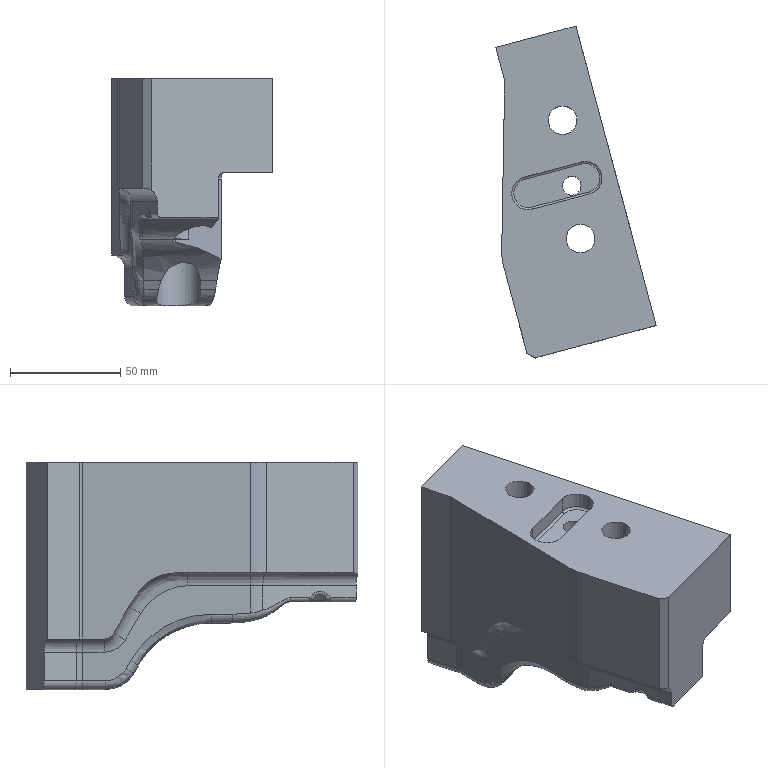Part | NX | features solid 2 | 1 solid | 77 faces | volume 452406 mm3 | cylinder 31 | plane 27 | spline 13 | torus 6 | commonest cylinder face diameters 8 x5 12 x5 6 x4 20 x3 2 x2 4 x2